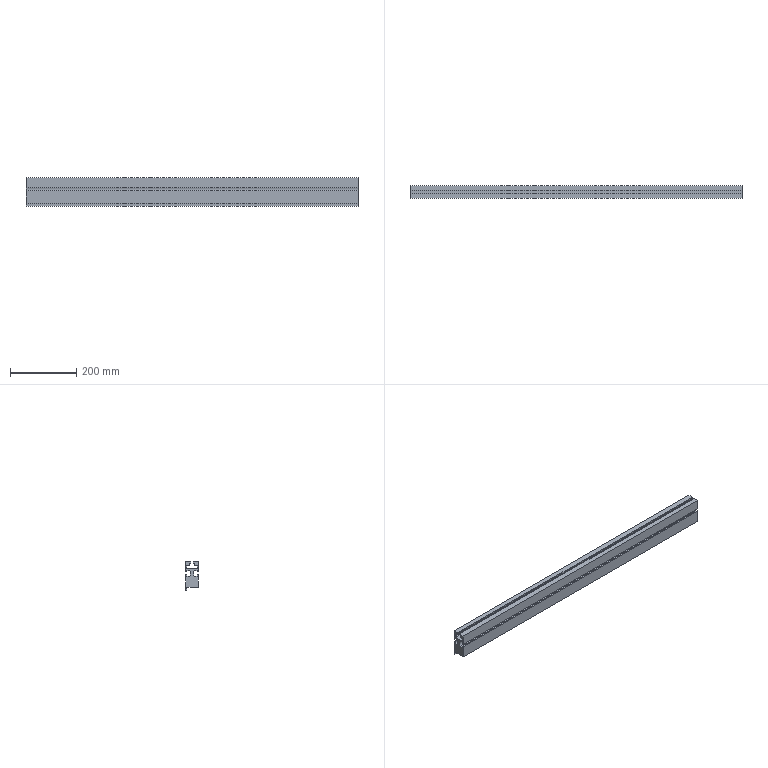Part | STEP file | 8000-001 | 1 solid | 42 faces | box 1000 x 38.9 x 86 mm | volume 2174515 mm3 | plane 34 | cylinder 8 | commonest cylinder face diameters 3.6 x6 29.068 x2